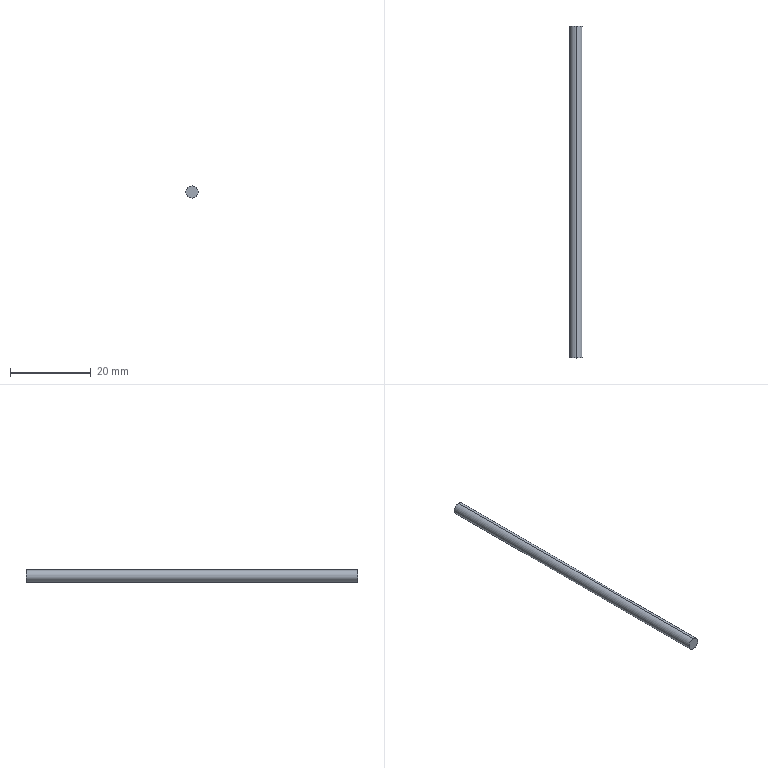Part | SolidWorks | features Extrusion 1 | 1 solid | 4 faces | box 3 x 82 x 3 mm | volume 579.624 mm3 | cylinder 2 | plane 2 | commonest cylinder face diameters 3 x2
STEP:
#1=CARTESIAN_POINT('',(0.,82.,1.5));
#2=VERTEX_POINT('',#1);
#3=CARTESIAN_POINT('',(0.,82.,-1.5));
#4=VERTEX_POINT('',#3);
#5=CARTESIAN_POINT('',(0.,82.,0.));
#6=DIRECTION('',(0.,1.,0.));
#7=DIRECTION('',(0.,0.,1.));
#8=AXIS2_PLACEMENT_3D('',#5,#6,#7);
#9=CIRCLE('',#8,1.5);
#10=EDGE_CURVE('',#2,#4,#9,.T.);
#11=ORIENTED_EDGE('',*,*,#10,.F.);
#12=CARTESIAN_POINT('',(0.,0.,1.5));
#13=VERTEX_POINT('',#12);
#14=CARTESIAN_POINT('',(0.,82.,1.5));
#15=DIRECTION('',(0.,-1.,0.));
#16=VECTOR('',#15,1000.);
#17=LINE('',#14,#16);
#18=EDGE_CURVE('',#2,#13,#17,.T.);
#19=ORIENTED_EDGE('',*,*,#18,.T.);
#20=CARTESIAN_POINT('',(0.,0.,-1.5));
#21=VERTEX_POINT('',#20);
#22=CARTESIAN_POINT('',(0.,0.,0.));
#23=DIRECTION('',(0.,1.,0.));
#24=DIRECTION('',(0.,0.,1.));
#25=AXIS2_PLACEMENT_3D('',#22,#23,#24);
#26=CIRCLE('',#25,1.5);
#27=EDGE_CURVE('',#13,#21,#26,.T.);
#28=ORIENTED_EDGE('',*,*,#27,.T.);
#29=CARTESIAN_POINT('',(0.,82.,-1.5));
#30=DIRECTION('',(0.,-1.,0.));
#31=VECTOR('',#30,1000.);
#32=LINE('',#29,#31);
#33=EDGE_CURVE('',#4,#21,#32,.T.);
#34=ORIENTED_EDGE('',*,*,#33,.F.);
#35=EDGE_LOOP('',(#11,#19,#28,#34));
#36=FACE_OUTER_BOUND('',#35,.T.);
#37=CARTESIAN_POINT('',(0.,82.,0.));
#38=DIRECTION('',(0.,-1.,0.));
#39=DIRECTION('',(0.,0.,-1.));
#40=AXIS2_PLACEMENT_3D('',#37,#38,#39);
#41=CYLINDRICAL_SURFACE('',#40,1.5);
#42=ADVANCED_FACE('',(#36),#41,.T.);
#43=ORIENTED_EDGE('',*,*,#18,.F.);
#44=CARTESIAN_POINT('',(0.,82.,0.));
#45=DIRECTION('',(0.,1.,0.));
#46=DIRECTION('',(0.,0.,1.));
#47=AXIS2_PLACEMENT_3D('',#44,#45,#46);
#48=CIRCLE('',#47,1.5);
#49=EDGE_CURVE('',#4,#2,#48,.T.);
#50=ORIENTED_EDGE('',*,*,#49,.F.);
#51=ORIENTED_EDGE('',*,*,#33,.T.);
#52=CARTESIAN_POINT('',(0.,0.,0.));
#53=DIRECTION('',(0.,1.,0.));
#54=DIRECTION('',(0.,0.,1.));
#55=AXIS2_PLACEMENT_3D('',#52,#53,#54);
#56=CIRCLE('',#55,1.5);
#57=EDGE_CURVE('',#21,#13,#56,.T.);
#58=ORIENTED_EDGE('',*,*,#57,.T.);
#59=EDGE_LOOP('',(#43,#50,#51,#58));
#60=FACE_OUTER_BOUND('',#59,.T.);
#61=CARTESIAN_POINT('',(0.,82.,0.));
#62=DIRECTION('',(0.,-1.,0.));
#63=DIRECTION('',(0.,0.,-1.));
#64=AXIS2_PLACEMENT_3D('',#61,#62,#63);
#65=CYLINDRICAL_SURFACE('',#64,1.5);
#66=ADVANCED_FACE('',(#60),#65,.T.);
#67=ORIENTED_EDGE('',*,*,#49,.T.);
#68=ORIENTED_EDGE('',*,*,#10,.T.);
#69=EDGE_LOOP('',(#67,#68));
#70=FACE_OUTER_BOUND('',#69,.T.);
#71=CARTESIAN_POINT('',(0.,82.,0.));
#72=DIRECTION('',(0.,1.,0.));
#73=DIRECTION('',(0.,0.,1.));
#74=AXIS2_PLACEMENT_3D('',#71,#72,#73);
#75=PLANE('',#74);
#76=ADVANCED_FACE('',(#70),#75,.T.);
#77=ORIENTED_EDGE('',*,*,#57,.F.);
#78=ORIENTED_EDGE('',*,*,#27,.F.);
#79=EDGE_LOOP('',(#77,#78));
#80=FACE_OUTER_BOUND('',#79,.T.);
#81=CARTESIAN_POINT('',(0.,0.,0.));
#82=DIRECTION('',(0.,1.,0.));
#83=DIRECTION('',(0.,0.,1.));
#84=AXIS2_PLACEMENT_3D('',#81,#82,#83);
#85=PLANE('',#84);
#86=ADVANCED_FACE('',(#80),#85,.F.);
#87=CLOSED_SHELL('',(#42,#66,#76,#86));
#88=MANIFOLD_SOLID_BREP('',#87);
#89=CARTESIAN_POINT('',(0.,0.,0.));
#90=DIRECTION('',(0.,0.,1.));
#91=DIRECTION('',(1.,0.,0.));
#92=AXIS2_PLACEMENT_3D('',#89,#90,#91);
#93=(LENGTH_UNIT()NAMED_UNIT(*)SI_UNIT(.MILLI.,.METRE.));
#94=UNCERTAINTY_MEASURE_WITH_UNIT(LENGTH_MEASURE(0.00001),#93,'','');
#95=(NAMED_UNIT(*)PLANE_ANGLE_UNIT()SI_UNIT($,.RADIAN.));
#96=(NAMED_UNIT(*)SI_UNIT($,.STERADIAN.)SOLID_ANGLE_UNIT());
#97=(GEOMETRIC_REPRESENTATION_CONTEXT(3)GLOBAL_UNCERTAINTY_ASSIGNED_CONTEXT((#94))GLOBAL_UNIT_ASSIGNED_CONTEXT((#93,#95,#96))REPRESENTATION_CONTEXT('',''));
#98=ADVANCED_BREP_SHAPE_REPRESENTATION('',(#88,#92),#97);